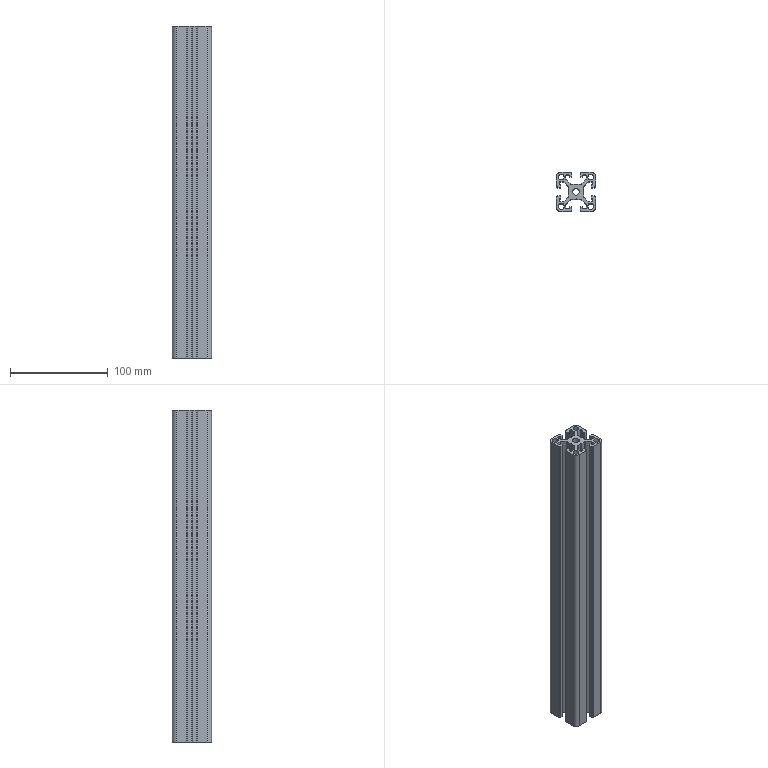Part | STEP file | HM-8-4040D-L340 | 1 solid | 176 faces | box 40 x 40 x 340 mm | volume 232783 mm3 | plane 90 | cylinder 86 | commonest cylinder face diameters 1 x40 0.4 x24 4 x8 6 x8 9 x4 6.8 x2